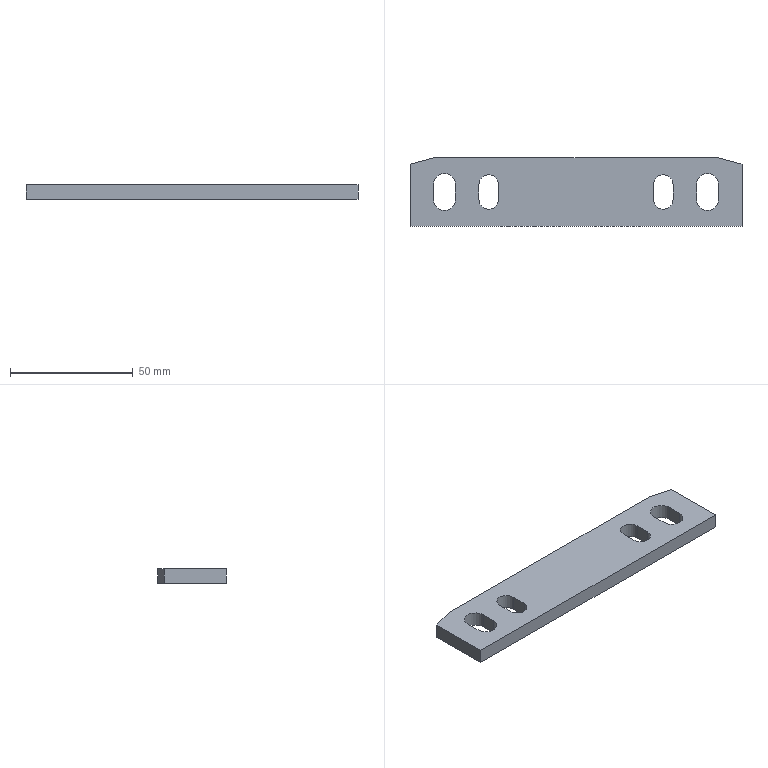Part | STEP file | gslz 2016.10.28-13_id1594_x_t | 1 solid | 24 faces | box 135 x 28 x 6 mm | volume 19929 mm3 | plane 16 | cylinder 8 | commonest cylinder face diameters 8 x4 9 x4